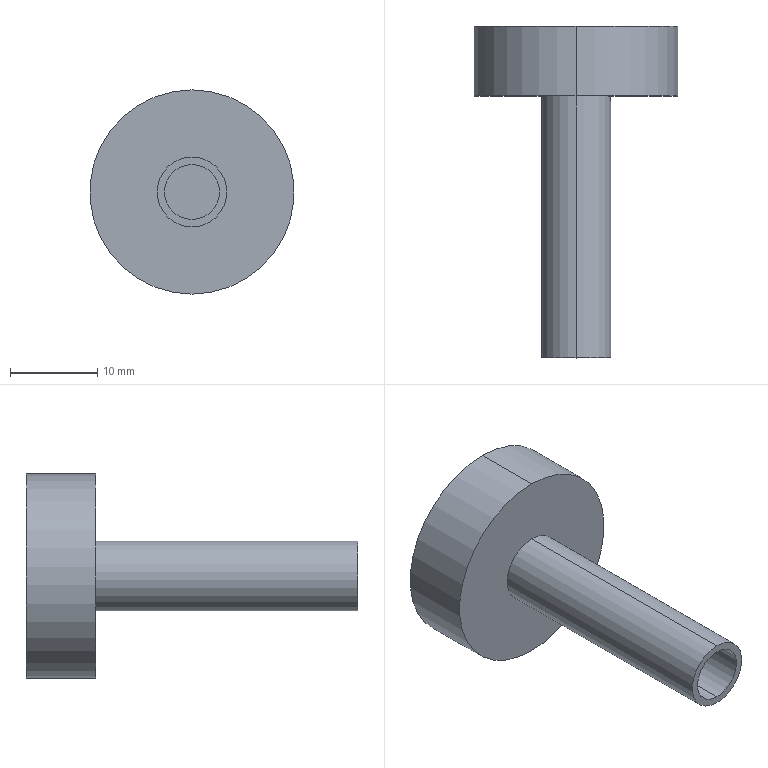Part | SolidWorks | features BaseBody 1 | 1 solid | 10 faces | box 23.4 x 38 x 23.4 mm | volume 4730 mm3 | cylinder 6 | plane 4 | commonest cylinder face diameters 6.3 x2 8 x2 23.4 x2
STEP:
#1=CARTESIAN_POINT('',(0.,-26.,4.));
#2=VERTEX_POINT('',#1);
#3=CARTESIAN_POINT('',(0.,-26.,-4.));
#4=VERTEX_POINT('',#3);
#5=CARTESIAN_POINT('',(0.,-26.,0.));
#6=DIRECTION('',(0.,1.,0.));
#7=DIRECTION('',(0.,0.,1.));
#8=AXIS2_PLACEMENT_3D('',#5,#6,#7);
#9=CIRCLE('',#8,4.);
#10=EDGE_CURVE('',#2,#4,#9,.T.);
#11=ORIENTED_EDGE('',*,*,#10,.T.);
#12=CARTESIAN_POINT('',(0.,4.,-4.));
#13=VERTEX_POINT('',#12);
#14=CARTESIAN_POINT('',(0.,-26.,-4.));
#15=DIRECTION('',(0.,1.,0.));
#16=VECTOR('',#15,1000.);
#17=LINE('',#14,#16);
#18=EDGE_CURVE('',#4,#13,#17,.T.);
#19=ORIENTED_EDGE('',*,*,#18,.T.);
#20=CARTESIAN_POINT('',(0.,4.,4.));
#21=VERTEX_POINT('',#20);
#22=CARTESIAN_POINT('',(0.,4.,0.));
#23=DIRECTION('',(0.,-1.,0.));
#24=DIRECTION('',(0.,0.,1.));
#25=AXIS2_PLACEMENT_3D('',#22,#23,#24);
#26=CIRCLE('',#25,4.);
#27=EDGE_CURVE('',#13,#21,#26,.T.);
#28=ORIENTED_EDGE('',*,*,#27,.T.);
#29=CARTESIAN_POINT('',(0.,-26.,4.));
#30=DIRECTION('',(0.,1.,0.));
#31=VECTOR('',#30,1000.);
#32=LINE('',#29,#31);
#33=EDGE_CURVE('',#2,#21,#32,.T.);
#34=ORIENTED_EDGE('',*,*,#33,.F.);
#35=EDGE_LOOP('',(#11,#19,#28,#34));
#36=FACE_OUTER_BOUND('',#35,.T.);
#37=CARTESIAN_POINT('',(0.,-26.,0.));
#38=DIRECTION('',(0.,1.,0.));
#39=DIRECTION('',(0.,0.,1.));
#40=AXIS2_PLACEMENT_3D('',#37,#38,#39);
#41=CYLINDRICAL_SURFACE('',#40,4.);
#42=ADVANCED_FACE('',(#36),#41,.T.);
#43=CARTESIAN_POINT('',(0.,-26.,3.15));
#44=VERTEX_POINT('',#43);
#45=CARTESIAN_POINT('',(0.,-26.,-3.15));
#46=VERTEX_POINT('',#45);
#47=CARTESIAN_POINT('',(0.,-26.,0.));
#48=DIRECTION('',(0.,-1.,0.));
#49=DIRECTION('',(0.,0.,1.));
#50=AXIS2_PLACEMENT_3D('',#47,#48,#49);
#51=CIRCLE('',#50,3.15);
#52=EDGE_CURVE('',#44,#46,#51,.T.);
#53=ORIENTED_EDGE('',*,*,#52,.T.);
#54=CARTESIAN_POINT('',(0.,-19.,-3.15));
#55=VERTEX_POINT('',#54);
#56=CARTESIAN_POINT('',(0.,-30.,-3.15));
#57=DIRECTION('',(0.,1.,0.));
#58=VECTOR('',#57,1000.);
#59=LINE('',#56,#58);
#60=EDGE_CURVE('',#46,#55,#59,.T.);
#61=ORIENTED_EDGE('',*,*,#60,.T.);
#62=CARTESIAN_POINT('',(0.,-19.,3.15));
#63=VERTEX_POINT('',#62);
#64=CARTESIAN_POINT('',(0.,-19.,0.));
#65=DIRECTION('',(0.,-1.,0.));
#66=DIRECTION('',(0.,0.,1.));
#67=AXIS2_PLACEMENT_3D('',#64,#65,#66);
#68=CIRCLE('',#67,3.15);
#69=EDGE_CURVE('',#63,#55,#68,.T.);
#70=ORIENTED_EDGE('',*,*,#69,.F.);
#71=CARTESIAN_POINT('',(0.,-30.,3.15));
#72=DIRECTION('',(0.,1.,0.));
#73=VECTOR('',#72,1000.);
#74=LINE('',#71,#73);
#75=EDGE_CURVE('',#44,#63,#74,.T.);
#76=ORIENTED_EDGE('',*,*,#75,.F.);
#77=EDGE_LOOP('',(#53,#61,#70,#76));
#78=FACE_OUTER_BOUND('',#77,.T.);
#79=CARTESIAN_POINT('',(0.,-30.,0.));
#80=DIRECTION('',(0.,1.,0.));
#81=DIRECTION('',(0.,0.,1.));
#82=AXIS2_PLACEMENT_3D('',#79,#80,#81);
#83=CYLINDRICAL_SURFACE('',#82,3.15);
#84=ADVANCED_FACE('',(#78),#83,.F.);
#85=CARTESIAN_POINT('',(0.,4.,11.7));
#86=VERTEX_POINT('',#85);
#87=CARTESIAN_POINT('',(0.,4.,-11.7));
#88=VERTEX_POINT('',#87);
#89=CARTESIAN_POINT('',(0.,4.,0.));
#90=DIRECTION('',(0.,1.,0.));
#91=DIRECTION('',(0.,0.,1.));
#92=AXIS2_PLACEMENT_3D('',#89,#90,#91);
#93=CIRCLE('',#92,11.7);
#94=EDGE_CURVE('',#86,#88,#93,.T.);
#95=ORIENTED_EDGE('',*,*,#94,.T.);
#96=CARTESIAN_POINT('',(0.,12.,-11.7));
#97=VERTEX_POINT('',#96);
#98=CARTESIAN_POINT('',(0.,4.,-11.7));
#99=DIRECTION('',(0.,1.,0.));
#100=VECTOR('',#99,1000.);
#101=LINE('',#98,#100);
#102=EDGE_CURVE('',#88,#97,#101,.T.);
#103=ORIENTED_EDGE('',*,*,#102,.T.);
#104=CARTESIAN_POINT('',(0.,12.,11.7));
#105=VERTEX_POINT('',#104);
#106=CARTESIAN_POINT('',(0.,12.,0.));
#107=DIRECTION('',(0.,-1.,0.));
#108=DIRECTION('',(0.,0.,1.));
#109=AXIS2_PLACEMENT_3D('',#106,#107,#108);
#110=CIRCLE('',#109,11.7);
#111=EDGE_CURVE('',#97,#105,#110,.T.);
#112=ORIENTED_EDGE('',*,*,#111,.T.);
#113=CARTESIAN_POINT('',(0.,4.,11.7));
#114=DIRECTION('',(0.,1.,0.));
#115=VECTOR('',#114,1000.);
#116=LINE('',#113,#115);
#117=EDGE_CURVE('',#86,#105,#116,.T.);
#118=ORIENTED_EDGE('',*,*,#117,.F.);
#119=EDGE_LOOP('',(#95,#103,#112,#118));
#120=FACE_OUTER_BOUND('',#119,.T.);
#121=CARTESIAN_POINT('',(0.,4.,0.));
#122=DIRECTION('',(0.,1.,0.));
#123=DIRECTION('',(0.,0.,1.));
#124=AXIS2_PLACEMENT_3D('',#121,#122,#123);
#125=CYLINDRICAL_SURFACE('',#124,11.7);
#126=ADVANCED_FACE('',(#120),#125,.T.);
#127=ORIENTED_EDGE('',*,*,#18,.F.);
#128=CARTESIAN_POINT('',(0.,-26.,0.));
#129=DIRECTION('',(0.,1.,0.));
#130=DIRECTION('',(0.,0.,1.));
#131=AXIS2_PLACEMENT_3D('',#128,#129,#130);
#132=CIRCLE('',#131,4.);
#133=EDGE_CURVE('',#4,#2,#132,.T.);
#134=ORIENTED_EDGE('',*,*,#133,.T.);
#135=ORIENTED_EDGE('',*,*,#33,.T.);
#136=CARTESIAN_POINT('',(0.,4.,0.));
#137=DIRECTION('',(0.,-1.,0.));
#138=DIRECTION('',(0.,0.,1.));
#139=AXIS2_PLACEMENT_3D('',#136,#137,#138);
#140=CIRCLE('',#139,4.);
#141=EDGE_CURVE('',#21,#13,#140,.T.);
#142=ORIENTED_EDGE('',*,*,#141,.T.);
#143=EDGE_LOOP('',(#127,#134,#135,#142));
#144=FACE_OUTER_BOUND('',#143,.T.);
#145=CARTESIAN_POINT('',(0.,-26.,0.));
#146=DIRECTION('',(0.,1.,0.));
#147=DIRECTION('',(0.,0.,1.));
#148=AXIS2_PLACEMENT_3D('',#145,#146,#147);
#149=CYLINDRICAL_SURFACE('',#148,4.);
#150=ADVANCED_FACE('',(#144),#149,.T.);
#151=ORIENTED_EDGE('',*,*,#52,.F.);
#152=CARTESIAN_POINT('',(0.,-26.,0.));
#153=DIRECTION('',(0.,-1.,0.));
#154=DIRECTION('',(0.,0.,1.));
#155=AXIS2_PLACEMENT_3D('',#152,#153,#154);
#156=CIRCLE('',#155,3.15);
#157=EDGE_CURVE('',#46,#44,#156,.T.);
#158=ORIENTED_EDGE('',*,*,#157,.F.);
#159=EDGE_LOOP('',(#151,#158));
#160=FACE_BOUND('',#159,.T.);
#161=ORIENTED_EDGE('',*,*,#10,.F.);
#162=ORIENTED_EDGE('',*,*,#133,.F.);
#163=EDGE_LOOP('',(#161,#162));
#164=FACE_OUTER_BOUND('',#163,.T.);
#165=CARTESIAN_POINT('',(0.,-26.,0.));
#166=DIRECTION('',(0.,1.,0.));
#167=DIRECTION('',(0.,0.,1.));
#168=AXIS2_PLACEMENT_3D('',#165,#166,#167);
#169=PLANE('',#168);
#170=ADVANCED_FACE('',(#160,#164),#169,.F.);
#171=ORIENTED_EDGE('',*,*,#141,.F.);
#172=ORIENTED_EDGE('',*,*,#27,.F.);
#173=EDGE_LOOP('',(#171,#172));
#174=FACE_BOUND('',#173,.T.);
#175=ORIENTED_EDGE('',*,*,#94,.F.);
#176=CARTESIAN_POINT('',(0.,4.,0.));
#177=DIRECTION('',(0.,1.,0.));
#178=DIRECTION('',(0.,0.,1.));
#179=AXIS2_PLACEMENT_3D('',#176,#177,#178);
#180=CIRCLE('',#179,11.7);
#181=EDGE_CURVE('',#88,#86,#180,.T.);
#182=ORIENTED_EDGE('',*,*,#181,.F.);
#183=EDGE_LOOP('',(#175,#182));
#184=FACE_OUTER_BOUND('',#183,.T.);
#185=CARTESIAN_POINT('',(0.,4.,0.));
#186=DIRECTION('',(0.,1.,0.));
#187=DIRECTION('',(0.,0.,1.));
#188=AXIS2_PLACEMENT_3D('',#185,#186,#187);
#189=PLANE('',#188);
#190=ADVANCED_FACE('',(#174,#184),#189,.F.);
#191=ORIENTED_EDGE('',*,*,#60,.F.);
#192=ORIENTED_EDGE('',*,*,#157,.T.);
#193=ORIENTED_EDGE('',*,*,#75,.T.);
#194=CARTESIAN_POINT('',(0.,-19.,0.));
#195=DIRECTION('',(0.,-1.,0.));
#196=DIRECTION('',(0.,0.,1.));
#197=AXIS2_PLACEMENT_3D('',#194,#195,#196);
#198=CIRCLE('',#197,3.15);
#199=EDGE_CURVE('',#55,#63,#198,.T.);
#200=ORIENTED_EDGE('',*,*,#199,.F.);
#201=EDGE_LOOP('',(#191,#192,#193,#200));
#202=FACE_OUTER_BOUND('',#201,.T.);
#203=CARTESIAN_POINT('',(0.,-30.,0.));
#204=DIRECTION('',(0.,1.,0.));
#205=DIRECTION('',(0.,0.,1.));
#206=AXIS2_PLACEMENT_3D('',#203,#204,#205);
#207=CYLINDRICAL_SURFACE('',#206,3.15);
#208=ADVANCED_FACE('',(#202),#207,.F.);
#209=ORIENTED_EDGE('',*,*,#102,.F.);
#210=ORIENTED_EDGE('',*,*,#181,.T.);
#211=ORIENTED_EDGE('',*,*,#117,.T.);
#212=CARTESIAN_POINT('',(0.,12.,0.));
#213=DIRECTION('',(0.,-1.,0.));
#214=DIRECTION('',(0.,0.,1.));
#215=AXIS2_PLACEMENT_3D('',#212,#213,#214);
#216=CIRCLE('',#215,11.7);
#217=EDGE_CURVE('',#105,#97,#216,.T.);
#218=ORIENTED_EDGE('',*,*,#217,.T.);
#219=EDGE_LOOP('',(#209,#210,#211,#218));
#220=FACE_OUTER_BOUND('',#219,.T.);
#221=CARTESIAN_POINT('',(0.,4.,0.));
#222=DIRECTION('',(0.,1.,0.));
#223=DIRECTION('',(0.,0.,1.));
#224=AXIS2_PLACEMENT_3D('',#221,#222,#223);
#225=CYLINDRICAL_SURFACE('',#224,11.7);
#226=ADVANCED_FACE('',(#220),#225,.T.);
#227=ORIENTED_EDGE('',*,*,#69,.T.);
#228=ORIENTED_EDGE('',*,*,#199,.T.);
#229=EDGE_LOOP('',(#227,#228));
#230=FACE_OUTER_BOUND('',#229,.T.);
#231=CARTESIAN_POINT('',(0.,-19.,0.));
#232=DIRECTION('',(0.,1.,0.));
#233=DIRECTION('',(0.,0.,1.));
#234=AXIS2_PLACEMENT_3D('',#231,#232,#233);
#235=PLANE('',#234);
#236=ADVANCED_FACE('',(#230),#235,.F.);
#237=ORIENTED_EDGE('',*,*,#217,.F.);
#238=ORIENTED_EDGE('',*,*,#111,.F.);
#239=EDGE_LOOP('',(#237,#238));
#240=FACE_OUTER_BOUND('',#239,.T.);
#241=CARTESIAN_POINT('',(0.,12.,0.));
#242=DIRECTION('',(0.,1.,0.));
#243=DIRECTION('',(0.,0.,1.));
#244=AXIS2_PLACEMENT_3D('',#241,#242,#243);
#245=PLANE('',#244);
#246=ADVANCED_FACE('',(#240),#245,.T.);
#247=CLOSED_SHELL('',(#42,#84,#126,#150,#170,#190,#208,#226,#236,#246));
#248=MANIFOLD_SOLID_BREP('',#247);
#249=CARTESIAN_POINT('',(0.,0.,0.));
#250=DIRECTION('',(0.,0.,1.));
#251=DIRECTION('',(1.,0.,0.));
#252=AXIS2_PLACEMENT_3D('',#249,#250,#251);
#253=(LENGTH_UNIT()NAMED_UNIT(*)SI_UNIT(.MILLI.,.METRE.));
#254=UNCERTAINTY_MEASURE_WITH_UNIT(LENGTH_MEASURE(0.00001),#253,'','');
#255=(NAMED_UNIT(*)PLANE_ANGLE_UNIT()SI_UNIT($,.RADIAN.));
#256=(NAMED_UNIT(*)SI_UNIT($,.STERADIAN.)SOLID_ANGLE_UNIT());
#257=(GEOMETRIC_REPRESENTATION_CONTEXT(3)GLOBAL_UNCERTAINTY_ASSIGNED_CONTEXT((#254))GLOBAL_UNIT_ASSIGNED_CONTEXT((#253,#255,#256))REPRESENTATION_CONTEXT('',''));
#258=ADVANCED_BREP_SHAPE_REPRESENTATION('',(#248,#252),#257);